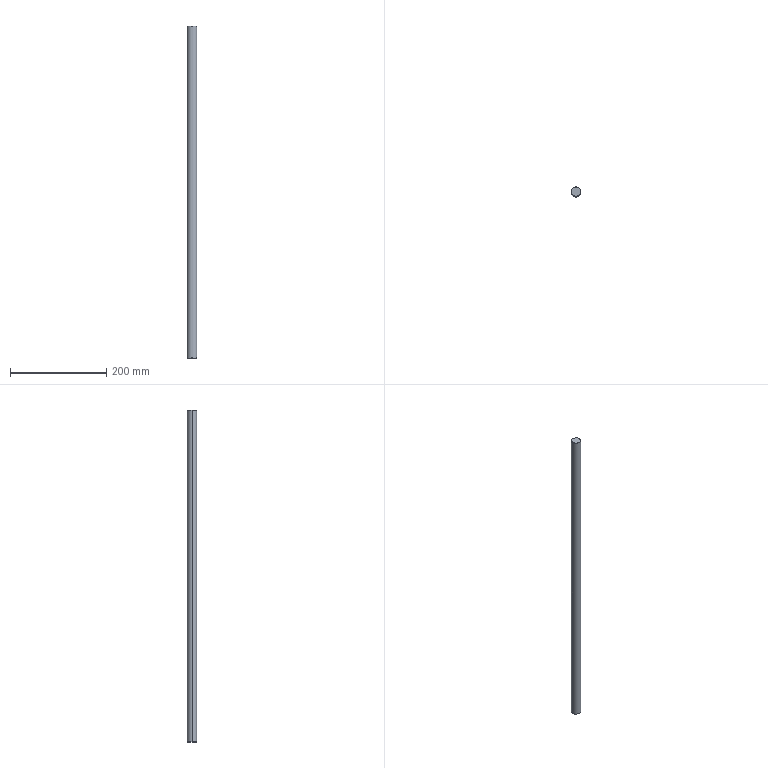Part | SolidWorks | features Chamfer 1, Extrusion 1 | 1 solid | 8 faces | box 20 x 20 x 690 mm | volume 216754 mm3 | cone 4 | cylinder 2 | plane 2 | commonest cylinder face diameters 20 x2
STEP:
#1=CARTESIAN_POINT('',(9.5,0.,345.));
#2=VERTEX_POINT('',#1);
#3=CARTESIAN_POINT('',(-9.5,0.,345.));
#4=VERTEX_POINT('',#3);
#5=CARTESIAN_POINT('',(0.,0.,345.));
#6=DIRECTION('',(0.,0.,1.));
#7=DIRECTION('',(1.,0.,0.));
#8=AXIS2_PLACEMENT_3D('',#5,#6,#7);
#9=CIRCLE('',#8,9.5);
#10=EDGE_CURVE('',#2,#4,#9,.T.);
#11=ORIENTED_EDGE('',*,*,#10,.F.);
#12=CARTESIAN_POINT('',(10.,0.,344.5));
#13=VERTEX_POINT('',#12);
#14=CARTESIAN_POINT('',(9.5,0.,345.));
#15=DIRECTION('',(0.7071,0.,-0.7071));
#16=VECTOR('',#15,1000.);
#17=LINE('',#14,#16);
#18=EDGE_CURVE('',#2,#13,#17,.T.);
#19=ORIENTED_EDGE('',*,*,#18,.T.);
#20=CARTESIAN_POINT('',(-10.,0.,344.5));
#21=VERTEX_POINT('',#20);
#22=CARTESIAN_POINT('',(0.,0.,344.5));
#23=DIRECTION('',(0.,0.,-1.));
#24=DIRECTION('',(1.,0.,0.));
#25=AXIS2_PLACEMENT_3D('',#22,#23,#24);
#26=CIRCLE('',#25,10.);
#27=EDGE_CURVE('',#21,#13,#26,.T.);
#28=ORIENTED_EDGE('',*,*,#27,.F.);
#29=CARTESIAN_POINT('',(-9.5,0.,345.));
#30=DIRECTION('',(-0.7071,0.,-0.7071));
#31=VECTOR('',#30,1000.);
#32=LINE('',#29,#31);
#33=EDGE_CURVE('',#4,#21,#32,.T.);
#34=ORIENTED_EDGE('',*,*,#33,.F.);
#35=EDGE_LOOP('',(#11,#19,#28,#34));
#36=FACE_OUTER_BOUND('',#35,.T.);
#37=CARTESIAN_POINT('',(0.,0.,345.));
#38=DIRECTION('',(0.,0.,-1.));
#39=DIRECTION('',(-1.,0.,0.));
#40=AXIS2_PLACEMENT_3D('',#37,#38,#39);
#41=CONICAL_SURFACE('',#40,9.5,0.7854);
#42=ADVANCED_FACE('',(#36),#41,.T.);
#43=CARTESIAN_POINT('',(-9.5,0.,-345.));
#44=VERTEX_POINT('',#43);
#45=CARTESIAN_POINT('',(9.5,0.,-345.));
#46=VERTEX_POINT('',#45);
#47=CARTESIAN_POINT('',(0.,0.,-345.));
#48=DIRECTION('',(0.,0.,-1.));
#49=DIRECTION('',(1.,0.,0.));
#50=AXIS2_PLACEMENT_3D('',#47,#48,#49);
#51=CIRCLE('',#50,9.5);
#52=EDGE_CURVE('',#44,#46,#51,.T.);
#53=ORIENTED_EDGE('',*,*,#52,.F.);
#54=CARTESIAN_POINT('',(-10.,0.,-344.5));
#55=VERTEX_POINT('',#54);
#56=CARTESIAN_POINT('',(-10.,0.,-344.5));
#57=DIRECTION('',(-0.7071,0.,0.7071));
#58=VECTOR('',#57,1000.);
#59=LINE('',#56,#58);
#60=EDGE_CURVE('',#44,#55,#59,.T.);
#61=ORIENTED_EDGE('',*,*,#60,.T.);
#62=CARTESIAN_POINT('',(10.,0.,-344.5));
#63=VERTEX_POINT('',#62);
#64=CARTESIAN_POINT('',(0.,0.,-344.5));
#65=DIRECTION('',(0.,0.,1.));
#66=DIRECTION('',(1.,0.,0.));
#67=AXIS2_PLACEMENT_3D('',#64,#65,#66);
#68=CIRCLE('',#67,10.);
#69=EDGE_CURVE('',#63,#55,#68,.T.);
#70=ORIENTED_EDGE('',*,*,#69,.F.);
#71=CARTESIAN_POINT('',(10.,0.,-344.5));
#72=DIRECTION('',(0.7071,0.,0.7071));
#73=VECTOR('',#72,1000.);
#74=LINE('',#71,#73);
#75=EDGE_CURVE('',#46,#63,#74,.T.);
#76=ORIENTED_EDGE('',*,*,#75,.F.);
#77=EDGE_LOOP('',(#53,#61,#70,#76));
#78=FACE_OUTER_BOUND('',#77,.T.);
#79=CARTESIAN_POINT('',(0.,0.,-344.5));
#80=DIRECTION('',(0.,0.,1.));
#81=DIRECTION('',(1.,0.,0.));
#82=AXIS2_PLACEMENT_3D('',#79,#80,#81);
#83=CONICAL_SURFACE('',#82,10.,0.7854);
#84=ADVANCED_FACE('',(#78),#83,.T.);
#85=ORIENTED_EDGE('',*,*,#27,.T.);
#86=CARTESIAN_POINT('',(10.,0.,345.));
#87=DIRECTION('',(0.,0.,-1.));
#88=VECTOR('',#87,1000.);
#89=LINE('',#86,#88);
#90=EDGE_CURVE('',#13,#63,#89,.T.);
#91=ORIENTED_EDGE('',*,*,#90,.T.);
#92=ORIENTED_EDGE('',*,*,#69,.T.);
#93=CARTESIAN_POINT('',(-10.,0.,345.));
#94=DIRECTION('',(0.,0.,-1.));
#95=VECTOR('',#94,1000.);
#96=LINE('',#93,#95);
#97=EDGE_CURVE('',#21,#55,#96,.T.);
#98=ORIENTED_EDGE('',*,*,#97,.F.);
#99=EDGE_LOOP('',(#85,#91,#92,#98));
#100=FACE_OUTER_BOUND('',#99,.T.);
#101=CARTESIAN_POINT('',(0.,0.,345.));
#102=DIRECTION('',(0.,0.,-1.));
#103=DIRECTION('',(-1.,0.,0.));
#104=AXIS2_PLACEMENT_3D('',#101,#102,#103);
#105=CYLINDRICAL_SURFACE('',#104,10.);
#106=ADVANCED_FACE('',(#100),#105,.T.);
#107=ORIENTED_EDGE('',*,*,#90,.F.);
#108=CARTESIAN_POINT('',(0.,0.,344.5));
#109=DIRECTION('',(0.,0.,-1.));
#110=DIRECTION('',(1.,0.,0.));
#111=AXIS2_PLACEMENT_3D('',#108,#109,#110);
#112=CIRCLE('',#111,10.);
#113=EDGE_CURVE('',#13,#21,#112,.T.);
#114=ORIENTED_EDGE('',*,*,#113,.T.);
#115=ORIENTED_EDGE('',*,*,#97,.T.);
#116=CARTESIAN_POINT('',(0.,0.,-344.5));
#117=DIRECTION('',(0.,0.,1.));
#118=DIRECTION('',(1.,0.,0.));
#119=AXIS2_PLACEMENT_3D('',#116,#117,#118);
#120=CIRCLE('',#119,10.);
#121=EDGE_CURVE('',#55,#63,#120,.T.);
#122=ORIENTED_EDGE('',*,*,#121,.T.);
#123=EDGE_LOOP('',(#107,#114,#115,#122));
#124=FACE_OUTER_BOUND('',#123,.T.);
#125=CARTESIAN_POINT('',(0.,0.,345.));
#126=DIRECTION('',(0.,0.,-1.));
#127=DIRECTION('',(-1.,0.,0.));
#128=AXIS2_PLACEMENT_3D('',#125,#126,#127);
#129=CYLINDRICAL_SURFACE('',#128,10.);
#130=ADVANCED_FACE('',(#124),#129,.T.);
#131=CARTESIAN_POINT('',(0.,0.,345.));
#132=DIRECTION('',(0.,0.,1.));
#133=DIRECTION('',(1.,0.,0.));
#134=AXIS2_PLACEMENT_3D('',#131,#132,#133);
#135=CIRCLE('',#134,9.5);
#136=EDGE_CURVE('',#4,#2,#135,.T.);
#137=ORIENTED_EDGE('',*,*,#136,.T.);
#138=ORIENTED_EDGE('',*,*,#10,.T.);
#139=EDGE_LOOP('',(#137,#138));
#140=FACE_OUTER_BOUND('',#139,.T.);
#141=CARTESIAN_POINT('',(0.,0.,345.));
#142=DIRECTION('',(0.,0.,1.));
#143=DIRECTION('',(1.,0.,0.));
#144=AXIS2_PLACEMENT_3D('',#141,#142,#143);
#145=PLANE('',#144);
#146=ADVANCED_FACE('',(#140),#145,.T.);
#147=CARTESIAN_POINT('',(0.,0.,-345.));
#148=DIRECTION('',(0.,0.,-1.));
#149=DIRECTION('',(1.,0.,0.));
#150=AXIS2_PLACEMENT_3D('',#147,#148,#149);
#151=CIRCLE('',#150,9.5);
#152=EDGE_CURVE('',#46,#44,#151,.T.);
#153=ORIENTED_EDGE('',*,*,#152,.T.);
#154=ORIENTED_EDGE('',*,*,#52,.T.);
#155=EDGE_LOOP('',(#153,#154));
#156=FACE_OUTER_BOUND('',#155,.T.);
#157=CARTESIAN_POINT('',(0.,0.,-345.));
#158=DIRECTION('',(0.,0.,1.));
#159=DIRECTION('',(1.,0.,0.));
#160=AXIS2_PLACEMENT_3D('',#157,#158,#159);
#161=PLANE('',#160);
#162=ADVANCED_FACE('',(#156),#161,.F.);
#163=ORIENTED_EDGE('',*,*,#60,.F.);
#164=ORIENTED_EDGE('',*,*,#152,.F.);
#165=ORIENTED_EDGE('',*,*,#75,.T.);
#166=ORIENTED_EDGE('',*,*,#121,.F.);
#167=EDGE_LOOP('',(#163,#164,#165,#166));
#168=FACE_OUTER_BOUND('',#167,.T.);
#169=CARTESIAN_POINT('',(0.,0.,-344.5));
#170=DIRECTION('',(0.,0.,1.));
#171=DIRECTION('',(1.,0.,0.));
#172=AXIS2_PLACEMENT_3D('',#169,#170,#171);
#173=CONICAL_SURFACE('',#172,10.,0.7854);
#174=ADVANCED_FACE('',(#168),#173,.T.);
#175=ORIENTED_EDGE('',*,*,#18,.F.);
#176=ORIENTED_EDGE('',*,*,#136,.F.);
#177=ORIENTED_EDGE('',*,*,#33,.T.);
#178=ORIENTED_EDGE('',*,*,#113,.F.);
#179=EDGE_LOOP('',(#175,#176,#177,#178));
#180=FACE_OUTER_BOUND('',#179,.T.);
#181=CARTESIAN_POINT('',(0.,0.,345.));
#182=DIRECTION('',(0.,0.,-1.));
#183=DIRECTION('',(-1.,0.,0.));
#184=AXIS2_PLACEMENT_3D('',#181,#182,#183);
#185=CONICAL_SURFACE('',#184,9.5,0.7854);
#186=ADVANCED_FACE('',(#180),#185,.T.);
#187=CLOSED_SHELL('',(#42,#84,#106,#130,#146,#162,#174,#186));
#188=MANIFOLD_SOLID_BREP('',#187);
#189=CARTESIAN_POINT('',(0.,0.,0.));
#190=DIRECTION('',(0.,0.,1.));
#191=DIRECTION('',(1.,0.,0.));
#192=AXIS2_PLACEMENT_3D('',#189,#190,#191);
#193=(LENGTH_UNIT()NAMED_UNIT(*)SI_UNIT(.MILLI.,.METRE.));
#194=UNCERTAINTY_MEASURE_WITH_UNIT(LENGTH_MEASURE(0.00001),#193,'','');
#195=(NAMED_UNIT(*)PLANE_ANGLE_UNIT()SI_UNIT($,.RADIAN.));
#196=(NAMED_UNIT(*)SI_UNIT($,.STERADIAN.)SOLID_ANGLE_UNIT());
#197=(GEOMETRIC_REPRESENTATION_CONTEXT(3)GLOBAL_UNCERTAINTY_ASSIGNED_CONTEXT((#194))GLOBAL_UNIT_ASSIGNED_CONTEXT((#193,#195,#196))REPRESENTATION_CONTEXT('',''));
#198=ADVANCED_BREP_SHAPE_REPRESENTATION('',(#188,#192),#197);